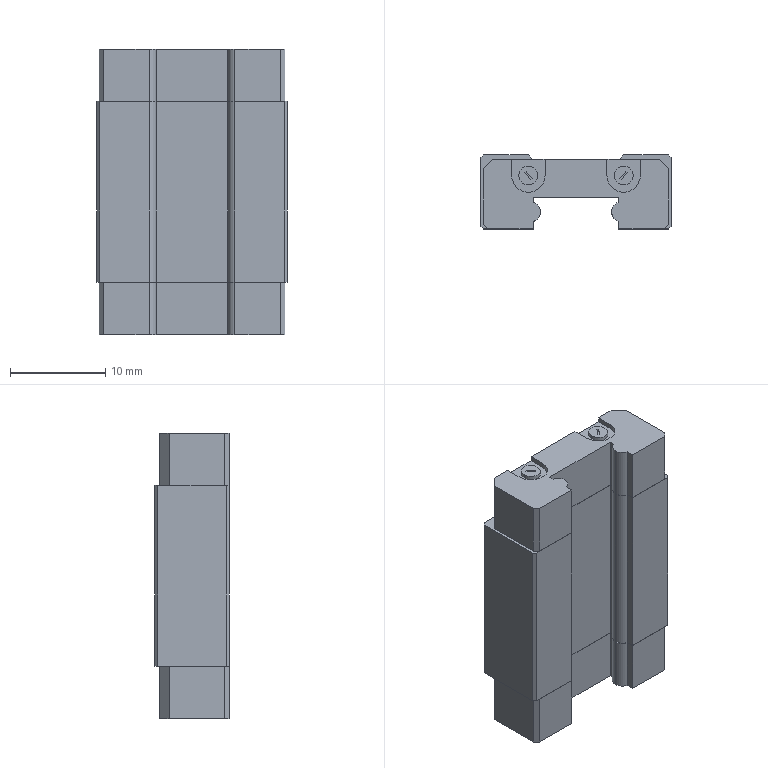Part | STEP file | SEZB10 | 1 solid | 167 faces | box 20 x 7.8 x 30 mm | volume 3504 mm3 | plane 116 | cylinder 35 | cone 16 | commonest cylinder face diameters 2.08 x9 2 x8 2.459 x8 1.68 x6 3.5 x4